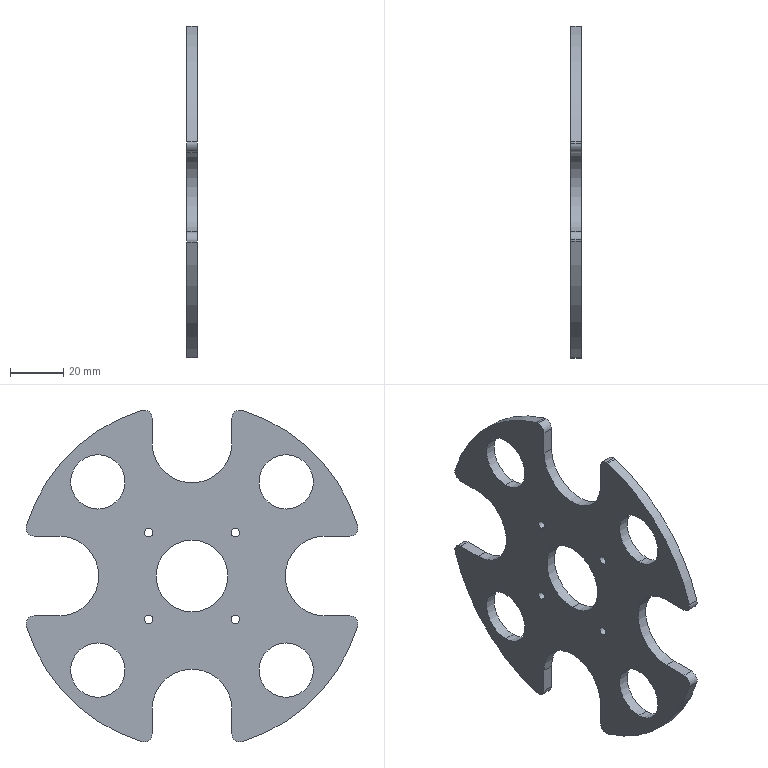Part | STEP file | Chuck wheel | 1 solid | 47 faces | box 4 x 124.659 x 124.659 mm | volume 32758 mm3 | cylinder 37 | plane 10 | commonest cylinder face diameters 6 x10 3.15 x8 20.4 x8 30 x5 130 x4 27 x2